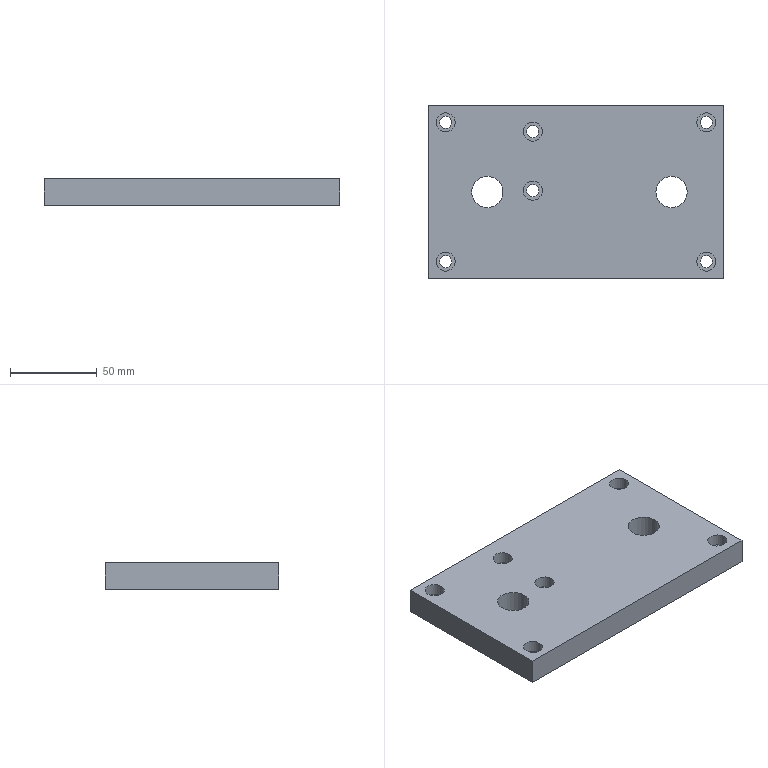Part | STEP file | solid 40 | 1 solid | 35 faces | box 170 x 100 x 15 mm | volume 236322 mm3 | cylinder 18 | plane 17 | commonest cylinder face diameters 7 x6 11 x6 10 x4 18 x2